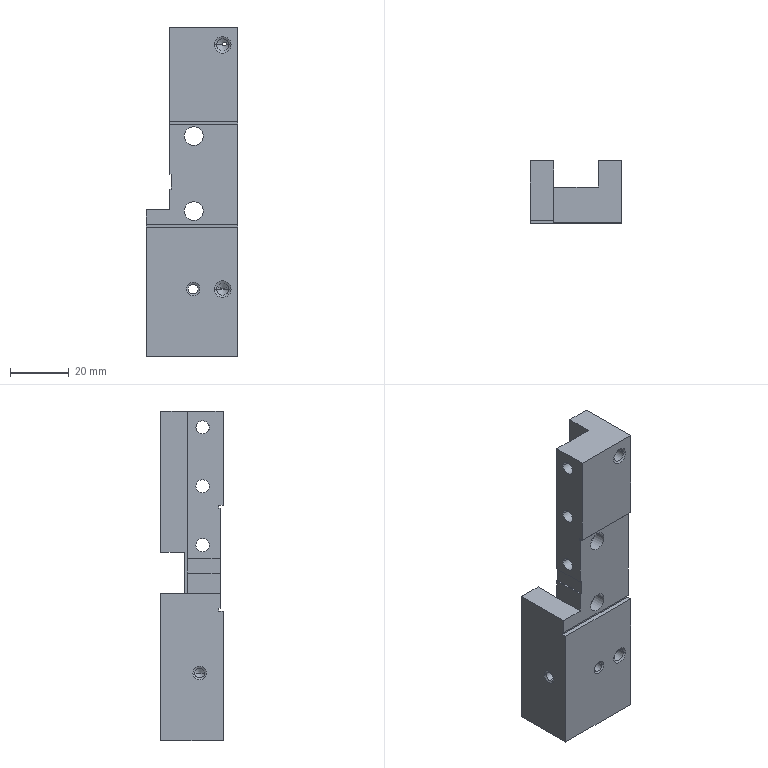Part | NX | 1 solid | 112 faces | box 31.2 x 21.2 x 112 mm | volume 42779 mm3 | cone 42 | cylinder 40 | plane 30 | commonest cylinder face diameters 3.3 x12 2.5 x8 4.5 x7 4.2 x5 6.4 x4 11 x4